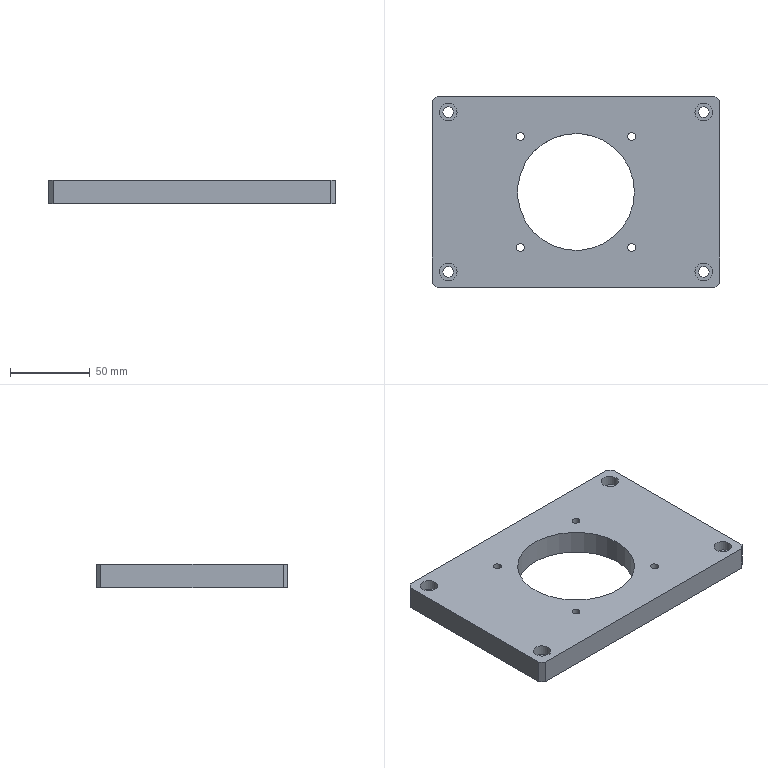Part | NX | 1 solid | 29 faces | box 180 x 120 x 15 mm | volume 255779 mm3 | plane 14 | cylinder 14 | cone 1 | commonest cylinder face diameters 5 x4 6.6 x4 11 x4 2.5 x1 73.2 x1
STEP:
#1=CARTESIAN_POINT('',(-87.,60.,7.5));
#2=VERTEX_POINT('',#1);
#3=CARTESIAN_POINT('',(-90.,57.,7.5));
#4=VERTEX_POINT('',#3);
#5=CARTESIAN_POINT('',(-73.5,73.5,7.5));
#6=DIRECTION('',(-0.7071,-0.7071,0.));
#7=VECTOR('',#6,1000.);
#8=LINE('',#5,#7);
#9=EDGE_CURVE('',#2,#4,#8,.T.);
#10=ORIENTED_EDGE('',*,*,#9,.F.);
#11=CARTESIAN_POINT('',(-87.,60.,-7.5));
#12=VERTEX_POINT('',#11);
#13=CARTESIAN_POINT('',(-87.,60.,7.5));
#14=DIRECTION('',(0.,0.,1.));
#15=VECTOR('',#14,1000.);
#16=LINE('',#13,#15);
#17=EDGE_CURVE('',#12,#2,#16,.T.);
#18=ORIENTED_EDGE('',*,*,#17,.F.);
#19=CARTESIAN_POINT('',(-90.,57.,-7.5));
#20=VERTEX_POINT('',#19);
#21=CARTESIAN_POINT('',(-90.,57.,-7.5));
#22=DIRECTION('',(0.7071,0.7071,0.));
#23=VECTOR('',#22,1000.);
#24=LINE('',#21,#23);
#25=EDGE_CURVE('',#20,#12,#24,.T.);
#26=ORIENTED_EDGE('',*,*,#25,.F.);
#27=CARTESIAN_POINT('',(-90.,57.,7.5));
#28=DIRECTION('',(0.,0.,-1.));
#29=VECTOR('',#28,1000.);
#30=LINE('',#27,#29);
#31=EDGE_CURVE('',#4,#20,#30,.T.);
#32=ORIENTED_EDGE('',*,*,#31,.F.);
#33=EDGE_LOOP('',(#10,#18,#26,#32));
#34=FACE_BOUND('',#33,.T.);
#35=CARTESIAN_POINT('',(-90.,57.,7.5));
#36=DIRECTION('',(0.7071,-0.7071,0.));
#37=DIRECTION('',(0.,0.,-1.));
#38=AXIS2_PLACEMENT_3D('',#35,#36,#37);
#39=PLANE('',#38);
#40=ADVANCED_FACE('',(#34),#39,.F.);
#41=CARTESIAN_POINT('',(90.,57.,7.5));
#42=VERTEX_POINT('',#41);
#43=CARTESIAN_POINT('',(87.,60.,7.5));
#44=VERTEX_POINT('',#43);
#45=CARTESIAN_POINT('',(73.5,73.5,7.5));
#46=DIRECTION('',(-0.7071,0.7071,0.));
#47=VECTOR('',#46,1000.);
#48=LINE('',#45,#47);
#49=EDGE_CURVE('',#42,#44,#48,.T.);
#50=ORIENTED_EDGE('',*,*,#49,.F.);
#51=CARTESIAN_POINT('',(90.,57.,-7.5));
#52=VERTEX_POINT('',#51);
#53=CARTESIAN_POINT('',(90.,57.,7.5));
#54=DIRECTION('',(0.,0.,1.));
#55=VECTOR('',#54,1000.);
#56=LINE('',#53,#55);
#57=EDGE_CURVE('',#52,#42,#56,.T.);
#58=ORIENTED_EDGE('',*,*,#57,.F.);
#59=CARTESIAN_POINT('',(87.,60.,-7.5));
#60=VERTEX_POINT('',#59);
#61=CARTESIAN_POINT('',(87.,60.,-7.5));
#62=DIRECTION('',(0.7071,-0.7071,0.));
#63=VECTOR('',#62,1000.);
#64=LINE('',#61,#63);
#65=EDGE_CURVE('',#60,#52,#64,.T.);
#66=ORIENTED_EDGE('',*,*,#65,.F.);
#67=CARTESIAN_POINT('',(87.,60.,7.5));
#68=DIRECTION('',(0.,0.,-1.));
#69=VECTOR('',#68,1000.);
#70=LINE('',#67,#69);
#71=EDGE_CURVE('',#44,#60,#70,.T.);
#72=ORIENTED_EDGE('',*,*,#71,.F.);
#73=EDGE_LOOP('',(#50,#58,#66,#72));
#74=FACE_BOUND('',#73,.T.);
#75=CARTESIAN_POINT('',(87.,60.,7.5));
#76=DIRECTION('',(-0.7071,-0.7071,0.));
#77=DIRECTION('',(0.,0.,-1.));
#78=AXIS2_PLACEMENT_3D('',#75,#76,#77);
#79=PLANE('',#78);
#80=ADVANCED_FACE('',(#74),#79,.F.);
#81=CARTESIAN_POINT('',(87.,-60.,7.5));
#82=VERTEX_POINT('',#81);
#83=CARTESIAN_POINT('',(90.,-57.,7.5));
#84=VERTEX_POINT('',#83);
#85=CARTESIAN_POINT('',(73.5,-73.5,7.5));
#86=DIRECTION('',(0.7071,0.7071,0.));
#87=VECTOR('',#86,1000.);
#88=LINE('',#85,#87);
#89=EDGE_CURVE('',#82,#84,#88,.T.);
#90=ORIENTED_EDGE('',*,*,#89,.F.);
#91=CARTESIAN_POINT('',(87.,-60.,-7.5));
#92=VERTEX_POINT('',#91);
#93=CARTESIAN_POINT('',(87.,-60.,7.5));
#94=DIRECTION('',(0.,0.,1.));
#95=VECTOR('',#94,1000.);
#96=LINE('',#93,#95);
#97=EDGE_CURVE('',#92,#82,#96,.T.);
#98=ORIENTED_EDGE('',*,*,#97,.F.);
#99=CARTESIAN_POINT('',(90.,-57.,-7.5));
#100=VERTEX_POINT('',#99);
#101=CARTESIAN_POINT('',(90.,-57.,-7.5));
#102=DIRECTION('',(-0.7071,-0.7071,0.));
#103=VECTOR('',#102,1000.);
#104=LINE('',#101,#103);
#105=EDGE_CURVE('',#100,#92,#104,.T.);
#106=ORIENTED_EDGE('',*,*,#105,.F.);
#107=CARTESIAN_POINT('',(90.,-57.,7.5));
#108=DIRECTION('',(0.,0.,-1.));
#109=VECTOR('',#108,1000.);
#110=LINE('',#107,#109);
#111=EDGE_CURVE('',#84,#100,#110,.T.);
#112=ORIENTED_EDGE('',*,*,#111,.F.);
#113=EDGE_LOOP('',(#90,#98,#106,#112));
#114=FACE_BOUND('',#113,.T.);
#115=CARTESIAN_POINT('',(90.,-57.,7.5));
#116=DIRECTION('',(-0.7071,0.7071,0.));
#117=DIRECTION('',(0.,0.,-1.));
#118=AXIS2_PLACEMENT_3D('',#115,#116,#117);
#119=PLANE('',#118);
#120=ADVANCED_FACE('',(#114),#119,.F.);
#121=CARTESIAN_POINT('',(-90.,-57.,7.5));
#122=VERTEX_POINT('',#121);
#123=CARTESIAN_POINT('',(-87.,-60.,7.5));
#124=VERTEX_POINT('',#123);
#125=CARTESIAN_POINT('',(-73.5,-73.5,7.5));
#126=DIRECTION('',(0.7071,-0.7071,0.));
#127=VECTOR('',#126,1000.);
#128=LINE('',#125,#127);
#129=EDGE_CURVE('',#122,#124,#128,.T.);
#130=ORIENTED_EDGE('',*,*,#129,.F.);
#131=CARTESIAN_POINT('',(-90.,-57.,-7.5));
#132=VERTEX_POINT('',#131);
#133=CARTESIAN_POINT('',(-90.,-57.,7.5));
#134=DIRECTION('',(0.,0.,1.));
#135=VECTOR('',#134,1000.);
#136=LINE('',#133,#135);
#137=EDGE_CURVE('',#132,#122,#136,.T.);
#138=ORIENTED_EDGE('',*,*,#137,.F.);
#139=CARTESIAN_POINT('',(-87.,-60.,-7.5));
#140=VERTEX_POINT('',#139);
#141=CARTESIAN_POINT('',(-87.,-60.,-7.5));
#142=DIRECTION('',(-0.7071,0.7071,0.));
#143=VECTOR('',#142,1000.);
#144=LINE('',#141,#143);
#145=EDGE_CURVE('',#140,#132,#144,.T.);
#146=ORIENTED_EDGE('',*,*,#145,.F.);
#147=CARTESIAN_POINT('',(-87.,-60.,7.5));
#148=DIRECTION('',(0.,0.,-1.));
#149=VECTOR('',#148,1000.);
#150=LINE('',#147,#149);
#151=EDGE_CURVE('',#124,#140,#150,.T.);
#152=ORIENTED_EDGE('',*,*,#151,.F.);
#153=EDGE_LOOP('',(#130,#138,#146,#152));
#154=FACE_BOUND('',#153,.T.);
#155=CARTESIAN_POINT('',(-87.,-60.,7.5));
#156=DIRECTION('',(0.7071,0.7071,0.));
#157=DIRECTION('',(0.,0.,-1.));
#158=AXIS2_PLACEMENT_3D('',#155,#156,#157);
#159=PLANE('',#158);
#160=ADVANCED_FACE('',(#154),#159,.F.);
#161=CARTESIAN_POINT('',(-85.5,50.,1.1));
#162=VERTEX_POINT('',#161);
#163=CARTESIAN_POINT('',(-80.,50.,1.1));
#164=DIRECTION('',(0.,0.,1.));
#165=DIRECTION('',(-1.,0.,0.));
#166=AXIS2_PLACEMENT_3D('',#163,#164,#165);
#167=CIRCLE('',#166,5.5);
#168=EDGE_CURVE('',#162,#162,#167,.T.);
#169=ORIENTED_EDGE('',*,*,#168,.T.);
#170=EDGE_LOOP('',(#169));
#171=FACE_BOUND('',#170,.T.);
#172=CARTESIAN_POINT('',(-83.3,50.,1.1));
#173=VERTEX_POINT('',#172);
#174=CARTESIAN_POINT('',(-80.,50.,1.1));
#175=DIRECTION('',(0.,0.,1.));
#176=DIRECTION('',(-1.,0.,0.));
#177=AXIS2_PLACEMENT_3D('',#174,#175,#176);
#178=CIRCLE('',#177,3.3);
#179=EDGE_CURVE('',#173,#173,#178,.T.);
#180=ORIENTED_EDGE('',*,*,#179,.F.);
#181=EDGE_LOOP('',(#180));
#182=FACE_BOUND('',#181,.T.);
#183=CARTESIAN_POINT('',(-76.7,-50.,1.1));
#184=DIRECTION('',(0.,0.,-1.));
#185=DIRECTION('',(-1.,0.,0.));
#186=AXIS2_PLACEMENT_3D('',#183,#184,#185);
#187=PLANE('',#186);
#188=ADVANCED_FACE('',(#171,#182),#187,.F.);
#189=CARTESIAN_POINT('',(74.5,50.,1.1));
#190=VERTEX_POINT('',#189);
#191=CARTESIAN_POINT('',(80.,50.,1.1));
#192=DIRECTION('',(0.,0.,1.));
#193=DIRECTION('',(-1.,0.,0.));
#194=AXIS2_PLACEMENT_3D('',#191,#192,#193);
#195=CIRCLE('',#194,5.5);
#196=EDGE_CURVE('',#190,#190,#195,.T.);
#197=ORIENTED_EDGE('',*,*,#196,.T.);
#198=EDGE_LOOP('',(#197));
#199=FACE_BOUND('',#198,.T.);
#200=CARTESIAN_POINT('',(76.7,50.,1.1));
#201=VERTEX_POINT('',#200);
#202=CARTESIAN_POINT('',(80.,50.,1.1));
#203=DIRECTION('',(0.,0.,1.));
#204=DIRECTION('',(-1.,0.,0.));
#205=AXIS2_PLACEMENT_3D('',#202,#203,#204);
#206=CIRCLE('',#205,3.3);
#207=EDGE_CURVE('',#201,#201,#206,.T.);
#208=ORIENTED_EDGE('',*,*,#207,.F.);
#209=EDGE_LOOP('',(#208));
#210=FACE_BOUND('',#209,.T.);
#211=CARTESIAN_POINT('',(-76.7,-50.,1.1));
#212=DIRECTION('',(0.,0.,-1.));
#213=DIRECTION('',(-1.,0.,0.));
#214=AXIS2_PLACEMENT_3D('',#211,#212,#213);
#215=PLANE('',#214);
#216=ADVANCED_FACE('',(#199,#210),#215,.F.);
#217=CARTESIAN_POINT('',(74.5,-50.,1.1));
#218=VERTEX_POINT('',#217);
#219=CARTESIAN_POINT('',(80.,-50.,1.1));
#220=DIRECTION('',(0.,0.,1.));
#221=DIRECTION('',(-1.,0.,0.));
#222=AXIS2_PLACEMENT_3D('',#219,#220,#221);
#223=CIRCLE('',#222,5.5);
#224=EDGE_CURVE('',#218,#218,#223,.T.);
#225=ORIENTED_EDGE('',*,*,#224,.T.);
#226=EDGE_LOOP('',(#225));
#227=FACE_BOUND('',#226,.T.);
#228=CARTESIAN_POINT('',(76.7,-50.,1.1));
#229=VERTEX_POINT('',#228);
#230=CARTESIAN_POINT('',(80.,-50.,1.1));
#231=DIRECTION('',(0.,0.,1.));
#232=DIRECTION('',(-1.,0.,0.));
#233=AXIS2_PLACEMENT_3D('',#230,#231,#232);
#234=CIRCLE('',#233,3.3);
#235=EDGE_CURVE('',#229,#229,#234,.T.);
#236=ORIENTED_EDGE('',*,*,#235,.F.);
#237=EDGE_LOOP('',(#236));
#238=FACE_BOUND('',#237,.T.);
#239=CARTESIAN_POINT('',(-76.7,-50.,1.1));
#240=DIRECTION('',(0.,0.,-1.));
#241=DIRECTION('',(-1.,0.,0.));
#242=AXIS2_PLACEMENT_3D('',#239,#240,#241);
#243=PLANE('',#242);
#244=ADVANCED_FACE('',(#227,#238),#243,.F.);
#245=CARTESIAN_POINT('',(-74.5,-50.,1.1));
#246=VERTEX_POINT('',#245);
#247=CARTESIAN_POINT('',(-80.,-50.,1.1));
#248=DIRECTION('',(0.,0.,1.));
#249=DIRECTION('',(1.,0.,0.));
#250=AXIS2_PLACEMENT_3D('',#247,#248,#249);
#251=CIRCLE('',#250,5.5);
#252=EDGE_CURVE('',#246,#246,#251,.T.);
#253=ORIENTED_EDGE('',*,*,#252,.T.);
#254=EDGE_LOOP('',(#253));
#255=FACE_BOUND('',#254,.T.);
#256=CARTESIAN_POINT('',(-76.7,-50.,1.1));
#257=VERTEX_POINT('',#256);
#258=CARTESIAN_POINT('',(-80.,-50.,1.1));
#259=DIRECTION('',(0.,0.,1.));
#260=DIRECTION('',(1.,0.,0.));
#261=AXIS2_PLACEMENT_3D('',#258,#259,#260);
#262=CIRCLE('',#261,3.3);
#263=EDGE_CURVE('',#257,#257,#262,.T.);
#264=ORIENTED_EDGE('',*,*,#263,.F.);
#265=EDGE_LOOP('',(#264));
#266=FACE_BOUND('',#265,.T.);
#267=CARTESIAN_POINT('',(-76.7,-50.,1.1));
#268=DIRECTION('',(0.,0.,-1.));
#269=DIRECTION('',(-1.,0.,0.));
#270=AXIS2_PLACEMENT_3D('',#267,#268,#269);
#271=PLANE('',#270);
#272=ADVANCED_FACE('',(#255,#266),#271,.F.);
#273=CARTESIAN_POINT('',(-90.,-60.,-7.5));
#274=DIRECTION('',(1.,0.,0.));
#275=VECTOR('',#274,1000.);
#276=LINE('',#273,#275);
#277=EDGE_CURVE('',#140,#92,#276,.T.);
#278=ORIENTED_EDGE('',*,*,#277,.F.);
#279=ORIENTED_EDGE('',*,*,#145,.T.);
#280=CARTESIAN_POINT('',(-90.,60.,-7.5));
#281=DIRECTION('',(0.,-1.,0.));
#282=VECTOR('',#281,1000.);
#283=LINE('',#280,#282);
#284=EDGE_CURVE('',#20,#132,#283,.T.);
#285=ORIENTED_EDGE('',*,*,#284,.F.);
#286=ORIENTED_EDGE('',*,*,#25,.T.);
#287=CARTESIAN_POINT('',(-90.,60.,-7.5));
#288=DIRECTION('',(-1.,0.,0.));
#289=VECTOR('',#288,1000.);
#290=LINE('',#287,#289);
#291=EDGE_CURVE('',#60,#12,#290,.T.);
#292=ORIENTED_EDGE('',*,*,#291,.F.);
#293=ORIENTED_EDGE('',*,*,#65,.T.);
#294=CARTESIAN_POINT('',(90.,60.,-7.5));
#295=DIRECTION('',(0.,1.,0.));
#296=VECTOR('',#295,1000.);
#297=LINE('',#294,#296);
#298=EDGE_CURVE('',#100,#52,#297,.T.);
#299=ORIENTED_EDGE('',*,*,#298,.F.);
#300=ORIENTED_EDGE('',*,*,#105,.T.);
#301=EDGE_LOOP('',(#278,#279,#285,#286,#292,#293,#299,#300));
#302=FACE_BOUND('',#301,.T.);
#303=CARTESIAN_POINT('',(36.6,0.,-7.5));
#304=VERTEX_POINT('',#303);
#305=CARTESIAN_POINT('',(0.,0.,-7.5));
#306=DIRECTION('',(0.,0.,1.));
#307=DIRECTION('',(1.,0.,0.));
#308=AXIS2_PLACEMENT_3D('',#305,#306,#307);
#309=CIRCLE('',#308,36.6);
#310=EDGE_CURVE('',#304,#304,#309,.T.);
#311=ORIENTED_EDGE('',*,*,#310,.T.);
#312=EDGE_LOOP('',(#311));
#313=FACE_BOUND('',#312,.T.);
#314=CARTESIAN_POINT('',(-76.7,-50.,-7.5));
#315=VERTEX_POINT('',#314);
#316=CARTESIAN_POINT('',(-80.,-50.,-7.5));
#317=DIRECTION('',(0.,0.,1.));
#318=DIRECTION('',(1.,0.,0.));
#319=AXIS2_PLACEMENT_3D('',#316,#317,#318);
#320=CIRCLE('',#319,3.3);
#321=EDGE_CURVE('',#315,#315,#320,.T.);
#322=ORIENTED_EDGE('',*,*,#321,.T.);
#323=EDGE_LOOP('',(#322));
#324=FACE_BOUND('',#323,.T.);
#325=CARTESIAN_POINT('',(83.3,-50.,-7.5));
#326=VERTEX_POINT('',#325);
#327=CARTESIAN_POINT('',(80.,-50.,-7.5));
#328=DIRECTION('',(0.,0.,1.));
#329=DIRECTION('',(1.,0.,0.));
#330=AXIS2_PLACEMENT_3D('',#327,#328,#329);
#331=CIRCLE('',#330,3.3);
#332=EDGE_CURVE('',#326,#326,#331,.T.);
#333=ORIENTED_EDGE('',*,*,#332,.T.);
#334=EDGE_LOOP('',(#333));
#335=FACE_BOUND('',#334,.T.);
#336=CARTESIAN_POINT('',(83.3,50.,-7.5));
#337=VERTEX_POINT('',#336);
#338=CARTESIAN_POINT('',(80.,50.,-7.5));
#339=DIRECTION('',(0.,0.,1.));
#340=DIRECTION('',(1.,0.,0.));
#341=AXIS2_PLACEMENT_3D('',#338,#339,#340);
#342=CIRCLE('',#341,3.3);
#343=EDGE_CURVE('',#337,#337,#342,.T.);
#344=ORIENTED_EDGE('',*,*,#343,.T.);
#345=EDGE_LOOP('',(#344));
#346=FACE_BOUND('',#345,.T.);
#347=CARTESIAN_POINT('',(-76.7,50.,-7.5));
#348=VERTEX_POINT('',#347);
#349=CARTESIAN_POINT('',(-80.,50.,-7.5));
#350=DIRECTION('',(0.,0.,1.));
#351=DIRECTION('',(1.,0.,0.));
#352=AXIS2_PLACEMENT_3D('',#349,#350,#351);
#353=CIRCLE('',#352,3.3);
#354=EDGE_CURVE('',#348,#348,#353,.T.);
#355=ORIENTED_EDGE('',*,*,#354,.T.);
#356=EDGE_LOOP('',(#355));
#357=FACE_BOUND('',#356,.T.);
#358=CARTESIAN_POINT('',(-32.3,-34.8,-7.5));
#359=VERTEX_POINT('',#358);
#360=CARTESIAN_POINT('',(-34.8,-34.8,-7.5));
#361=DIRECTION('',(0.,0.,1.));
#362=DIRECTION('',(1.,0.,0.));
#363=AXIS2_PLACEMENT_3D('',#360,#361,#362);
#364=CIRCLE('',#363,2.5);
#365=EDGE_CURVE('',#359,#359,#364,.T.);
#366=ORIENTED_EDGE('',*,*,#365,.T.);
#367=EDGE_LOOP('',(#366));
#368=FACE_BOUND('',#367,.T.);
#369=CARTESIAN_POINT('',(37.3,-34.8,-7.5));
#370=VERTEX_POINT('',#369);
#371=CARTESIAN_POINT('',(34.8,-34.8,-7.5));
#372=DIRECTION('',(0.,0.,1.));
#373=DIRECTION('',(1.,0.,0.));
#374=AXIS2_PLACEMENT_3D('',#371,#372,#373);
#375=CIRCLE('',#374,2.5);
#376=EDGE_CURVE('',#370,#370,#375,.T.);
#377=ORIENTED_EDGE('',*,*,#376,.T.);
#378=EDGE_LOOP('',(#377));
#379=FACE_BOUND('',#378,.T.);
#380=CARTESIAN_POINT('',(37.3,34.8,-7.5));
#381=VERTEX_POINT('',#380);
#382=CARTESIAN_POINT('',(34.8,34.8,-7.5));
#383=DIRECTION('',(0.,0.,1.));
#384=DIRECTION('',(1.,0.,0.));
#385=AXIS2_PLACEMENT_3D('',#382,#383,#384);
#386=CIRCLE('',#385,2.5);
#387=EDGE_CURVE('',#381,#381,#386,.T.);
#388=ORIENTED_EDGE('',*,*,#387,.T.);
#389=EDGE_LOOP('',(#388));
#390=FACE_BOUND('',#389,.T.);
#391=CARTESIAN_POINT('',(-32.3,34.8,-7.5));
#392=VERTEX_POINT('',#391);
#393=CARTESIAN_POINT('',(-34.8,34.8,-7.5));
#394=DIRECTION('',(0.,0.,1.));
#395=DIRECTION('',(1.,0.,0.));
#396=AXIS2_PLACEMENT_3D('',#393,#394,#395);
#397=CIRCLE('',#396,2.5);
#398=EDGE_CURVE('',#392,#392,#397,.T.);
#399=ORIENTED_EDGE('',*,*,#398,.T.);
#400=EDGE_LOOP('',(#399));
#401=FACE_BOUND('',#400,.T.);
#402=CARTESIAN_POINT('',(0.,0.,-7.5));
#403=DIRECTION('',(0.,0.,1.));
#404=DIRECTION('',(1.,0.,0.));
#405=AXIS2_PLACEMENT_3D('',#402,#403,#404);
#406=PLANE('',#405);
#407=ADVANCED_FACE('',(#302,#313,#324,#335,#346,#357,#368,#379,#390,#401),#406,.F.);
#408=CARTESIAN_POINT('',(-90.,60.,7.5));
#409=DIRECTION('',(0.,-1.,0.));
#410=VECTOR('',#409,1000.);
#411=LINE('',#408,#410);
#412=EDGE_CURVE('',#4,#122,#411,.T.);
#413=ORIENTED_EDGE('',*,*,#412,.T.);
#414=ORIENTED_EDGE('',*,*,#129,.T.);
#415=CARTESIAN_POINT('',(-90.,-60.,7.5));
#416=DIRECTION('',(1.,0.,0.));
#417=VECTOR('',#416,1000.);
#418=LINE('',#415,#417);
#419=EDGE_CURVE('',#124,#82,#418,.T.);
#420=ORIENTED_EDGE('',*,*,#419,.T.);
#421=ORIENTED_EDGE('',*,*,#89,.T.);
#422=CARTESIAN_POINT('',(90.,60.,7.5));
#423=DIRECTION('',(0.,1.,0.));
#424=VECTOR('',#423,1000.);
#425=LINE('',#422,#424);
#426=EDGE_CURVE('',#84,#42,#425,.T.);
#427=ORIENTED_EDGE('',*,*,#426,.T.);
#428=ORIENTED_EDGE('',*,*,#49,.T.);
#429=CARTESIAN_POINT('',(-90.,60.,7.5));
#430=DIRECTION('',(-1.,0.,0.));
#431=VECTOR('',#430,1000.);
#432=LINE('',#429,#431);
#433=EDGE_CURVE('',#44,#2,#432,.T.);
#434=ORIENTED_EDGE('',*,*,#433,.T.);
#435=ORIENTED_EDGE('',*,*,#9,.T.);
#436=EDGE_LOOP('',(#413,#414,#420,#421,#427,#428,#434,#435));
#437=FACE_BOUND('',#436,.T.);
#438=CARTESIAN_POINT('',(36.6,0.,7.5));
#439=VERTEX_POINT('',#438);
#440=CARTESIAN_POINT('',(0.,0.,7.5));
#441=DIRECTION('',(0.,0.,1.));
#442=DIRECTION('',(1.,0.,0.));
#443=AXIS2_PLACEMENT_3D('',#440,#441,#442);
#444=CIRCLE('',#443,36.6);
#445=EDGE_CURVE('',#439,#439,#444,.T.);
#446=ORIENTED_EDGE('',*,*,#445,.F.);
#447=EDGE_LOOP('',(#446));
#448=FACE_BOUND('',#447,.T.);
#449=CARTESIAN_POINT('',(-74.5,-50.,7.5));
#450=VERTEX_POINT('',#449);
#451=CARTESIAN_POINT('',(-80.,-50.,7.5));
#452=DIRECTION('',(0.,0.,1.));
#453=DIRECTION('',(1.,0.,0.));
#454=AXIS2_PLACEMENT_3D('',#451,#452,#453);
#455=CIRCLE('',#454,5.5);
#456=EDGE_CURVE('',#450,#450,#455,.T.);
#457=ORIENTED_EDGE('',*,*,#456,.F.);
#458=EDGE_LOOP('',(#457));
#459=FACE_BOUND('',#458,.T.);
#460=CARTESIAN_POINT('',(85.5,-50.,7.5));
#461=VERTEX_POINT('',#460);
#462=CARTESIAN_POINT('',(80.,-50.,7.5));
#463=DIRECTION('',(0.,0.,1.));
#464=DIRECTION('',(1.,0.,0.));
#465=AXIS2_PLACEMENT_3D('',#462,#463,#464);
#466=CIRCLE('',#465,5.5);
#467=EDGE_CURVE('',#461,#461,#466,.T.);
#468=ORIENTED_EDGE('',*,*,#467,.F.);
#469=EDGE_LOOP('',(#468));
#470=FACE_BOUND('',#469,.T.);
#471=CARTESIAN_POINT('',(85.5,50.,7.5));
#472=VERTEX_POINT('',#471);
#473=CARTESIAN_POINT('',(80.,50.,7.5));
#474=DIRECTION('',(0.,0.,1.));
#475=DIRECTION('',(1.,0.,0.));
#476=AXIS2_PLACEMENT_3D('',#473,#474,#475);
#477=CIRCLE('',#476,5.5);
#478=EDGE_CURVE('',#472,#472,#477,.T.);
#479=ORIENTED_EDGE('',*,*,#478,.F.);
#480=EDGE_LOOP('',(#479));
#481=FACE_BOUND('',#480,.T.);
#482=CARTESIAN_POINT('',(-74.5,50.,7.5));
#483=VERTEX_POINT('',#482);
#484=CARTESIAN_POINT('',(-80.,50.,7.5));
#485=DIRECTION('',(0.,0.,1.));
#486=DIRECTION('',(1.,0.,0.));
#487=AXIS2_PLACEMENT_3D('',#484,#485,#486);
#488=CIRCLE('',#487,5.5);
#489=EDGE_CURVE('',#483,#483,#488,.T.);
#490=ORIENTED_EDGE('',*,*,#489,.F.);
#491=EDGE_LOOP('',(#490));
#492=FACE_BOUND('',#491,.T.);
#493=CARTESIAN_POINT('',(-32.3,-34.8,7.5));
#494=VERTEX_POINT('',#493);
#495=CARTESIAN_POINT('',(-34.8,-34.8,7.5));
#496=DIRECTION('',(0.,0.,1.));
#497=DIRECTION('',(1.,0.,0.));
#498=AXIS2_PLACEMENT_3D('',#495,#496,#497);
#499=CIRCLE('',#498,2.5);
#500=EDGE_CURVE('',#494,#494,#499,.T.);
#501=ORIENTED_EDGE('',*,*,#500,.F.);
#502=EDGE_LOOP('',(#501));
#503=FACE_BOUND('',#502,.T.);
#504=CARTESIAN_POINT('',(37.3,-34.8,7.5));
#505=VERTEX_POINT('',#504);
#506=CARTESIAN_POINT('',(34.8,-34.8,7.5));
#507=DIRECTION('',(0.,0.,1.));
#508=DIRECTION('',(1.,0.,0.));
#509=AXIS2_PLACEMENT_3D('',#506,#507,#508);
#510=CIRCLE('',#509,2.5);
#511=EDGE_CURVE('',#505,#505,#510,.T.);
#512=ORIENTED_EDGE('',*,*,#511,.F.);
#513=EDGE_LOOP('',(#512));
#514=FACE_BOUND('',#513,.T.);
#515=CARTESIAN_POINT('',(37.3,34.8,7.5));
#516=VERTEX_POINT('',#515);
#517=CARTESIAN_POINT('',(34.8,34.8,7.5));
#518=DIRECTION('',(0.,0.,1.));
#519=DIRECTION('',(1.,0.,0.));
#520=AXIS2_PLACEMENT_3D('',#517,#518,#519);
#521=CIRCLE('',#520,2.5);
#522=EDGE_CURVE('',#516,#516,#521,.T.);
#523=ORIENTED_EDGE('',*,*,#522,.F.);
#524=EDGE_LOOP('',(#523));
#525=FACE_BOUND('',#524,.T.);
#526=CARTESIAN_POINT('',(-32.3,34.8,7.5));
#527=VERTEX_POINT('',#526);
#528=CARTESIAN_POINT('',(-34.8,34.8,7.5));
#529=DIRECTION('',(0.,0.,1.));
#530=DIRECTION('',(1.,0.,0.));
#531=AXIS2_PLACEMENT_3D('',#528,#529,#530);
#532=CIRCLE('',#531,2.5);
#533=EDGE_CURVE('',#527,#527,#532,.T.);
#534=ORIENTED_EDGE('',*,*,#533,.F.);
#535=EDGE_LOOP('',(#534));
#536=FACE_BOUND('',#535,.T.);
#537=CARTESIAN_POINT('',(0.,0.,7.5));
#538=DIRECTION('',(0.,0.,1.));
#539=DIRECTION('',(1.,0.,0.));
#540=AXIS2_PLACEMENT_3D('',#537,#538,#539);
#541=PLANE('',#540);
#542=ADVANCED_FACE('',(#437,#448,#459,#470,#481,#492,#503,#514,#525,#536),#541,.T.);
#543=ORIENTED_EDGE('',*,*,#419,.F.);
#544=ORIENTED_EDGE('',*,*,#151,.T.);
#545=ORIENTED_EDGE('',*,*,#277,.T.);
#546=ORIENTED_EDGE('',*,*,#97,.T.);
#547=EDGE_LOOP('',(#543,#544,#545,#546));
#548=FACE_BOUND('',#547,.T.);
#549=CARTESIAN_POINT('',(-90.,-60.,7.5));
#550=DIRECTION('',(0.,1.,0.));
#551=DIRECTION('',(0.,0.,1.));
#552=AXIS2_PLACEMENT_3D('',#549,#550,#551);
#553=PLANE('',#552);
#554=ADVANCED_FACE('',(#548),#553,.F.);
#555=ORIENTED_EDGE('',*,*,#284,.T.);
#556=ORIENTED_EDGE('',*,*,#137,.T.);
#557=ORIENTED_EDGE('',*,*,#412,.F.);
#558=ORIENTED_EDGE('',*,*,#31,.T.);
#559=EDGE_LOOP('',(#555,#556,#557,#558));
#560=FACE_BOUND('',#559,.T.);
#561=CARTESIAN_POINT('',(-90.,60.,7.5));
#562=DIRECTION('',(1.,0.,0.));
#563=DIRECTION('',(0.,1.,0.));
#564=AXIS2_PLACEMENT_3D('',#561,#562,#563);
#565=PLANE('',#564);
#566=ADVANCED_FACE('',(#560),#565,.F.);
#567=ORIENTED_EDGE('',*,*,#433,.F.);
#568=ORIENTED_EDGE('',*,*,#71,.T.);
#569=ORIENTED_EDGE('',*,*,#291,.T.);
#570=ORIENTED_EDGE('',*,*,#17,.T.);
#571=EDGE_LOOP('',(#567,#568,#569,#570));
#572=FACE_BOUND('',#571,.T.);
#573=CARTESIAN_POINT('',(-15.5,60.,1.25));
#574=VERTEX_POINT('',#573);
#575=CARTESIAN_POINT('',(-15.5,60.,0.));
#576=DIRECTION('',(0.,1.,0.));
#577=DIRECTION('',(0.,0.,1.));
#578=AXIS2_PLACEMENT_3D('',#575,#576,#577);
#579=CIRCLE('',#578,1.25);
#580=EDGE_CURVE('',#574,#574,#579,.T.);
#581=ORIENTED_EDGE('',*,*,#580,.F.);
#582=EDGE_LOOP('',(#581));
#583=FACE_BOUND('',#582,.T.);
#584=CARTESIAN_POINT('',(-90.,60.,7.5));
#585=DIRECTION('',(0.,-1.,0.));
#586=DIRECTION('',(0.,0.,-1.));
#587=AXIS2_PLACEMENT_3D('',#584,#585,#586);
#588=PLANE('',#587);
#589=ADVANCED_FACE('',(#572,#583),#588,.F.);
#590=ORIENTED_EDGE('',*,*,#426,.F.);
#591=ORIENTED_EDGE('',*,*,#111,.T.);
#592=ORIENTED_EDGE('',*,*,#298,.T.);
#593=ORIENTED_EDGE('',*,*,#57,.T.);
#594=EDGE_LOOP('',(#590,#591,#592,#593));
#595=FACE_BOUND('',#594,.T.);
#596=CARTESIAN_POINT('',(90.,60.,7.5));
#597=DIRECTION('',(-1.,0.,0.));
#598=DIRECTION('',(0.,-1.,0.));
#599=AXIS2_PLACEMENT_3D('',#596,#597,#598);
#600=PLANE('',#599);
#601=ADVANCED_FACE('',(#595),#600,.F.);
#602=ORIENTED_EDGE('',*,*,#310,.F.);
#603=EDGE_LOOP('',(#602));
#604=FACE_BOUND('',#603,.T.);
#605=ORIENTED_EDGE('',*,*,#445,.T.);
#606=EDGE_LOOP('',(#605));
#607=FACE_BOUND('',#606,.T.);
#608=CARTESIAN_POINT('',(0.,0.,-7.5));
#609=DIRECTION('',(0.,0.,1.));
#610=DIRECTION('',(1.,0.,0.));
#611=AXIS2_PLACEMENT_3D('',#608,#609,#610);
#612=CYLINDRICAL_SURFACE('',#611,36.6);
#613=ADVANCED_FACE('',(#604,#607),#612,.F.);
#614=ORIENTED_EDGE('',*,*,#321,.F.);
#615=EDGE_LOOP('',(#614));
#616=FACE_BOUND('',#615,.T.);
#617=ORIENTED_EDGE('',*,*,#263,.T.);
#618=EDGE_LOOP('',(#617));
#619=FACE_BOUND('',#618,.T.);
#620=CARTESIAN_POINT('',(-80.,-50.,7.5));
#621=DIRECTION('',(0.,0.,1.));
#622=DIRECTION('',(1.,0.,0.));
#623=AXIS2_PLACEMENT_3D('',#620,#621,#622);
#624=CYLINDRICAL_SURFACE('',#623,3.3);
#625=ADVANCED_FACE('',(#616,#619),#624,.F.);
#626=ORIENTED_EDGE('',*,*,#252,.F.);
#627=EDGE_LOOP('',(#626));
#628=FACE_BOUND('',#627,.T.);
#629=ORIENTED_EDGE('',*,*,#456,.T.);
#630=EDGE_LOOP('',(#629));
#631=FACE_BOUND('',#630,.T.);
#632=CARTESIAN_POINT('',(-80.,-50.,7.5));
#633=DIRECTION('',(0.,0.,1.));
#634=DIRECTION('',(1.,0.,0.));
#635=AXIS2_PLACEMENT_3D('',#632,#633,#634);
#636=CYLINDRICAL_SURFACE('',#635,5.5);
#637=ADVANCED_FACE('',(#628,#631),#636,.F.);
#638=ORIENTED_EDGE('',*,*,#332,.F.);
#639=EDGE_LOOP('',(#638));
#640=FACE_BOUND('',#639,.T.);
#641=ORIENTED_EDGE('',*,*,#235,.T.);
#642=EDGE_LOOP('',(#641));
#643=FACE_BOUND('',#642,.T.);
#644=CARTESIAN_POINT('',(80.,-50.,7.5));
#645=DIRECTION('',(0.,0.,1.));
#646=DIRECTION('',(1.,0.,0.));
#647=AXIS2_PLACEMENT_3D('',#644,#645,#646);
#648=CYLINDRICAL_SURFACE('',#647,3.3);
#649=ADVANCED_FACE('',(#640,#643),#648,.F.);
#650=ORIENTED_EDGE('',*,*,#224,.F.);
#651=EDGE_LOOP('',(#650));
#652=FACE_BOUND('',#651,.T.);
#653=ORIENTED_EDGE('',*,*,#467,.T.);
#654=EDGE_LOOP('',(#653));
#655=FACE_BOUND('',#654,.T.);
#656=CARTESIAN_POINT('',(80.,-50.,7.5));
#657=DIRECTION('',(0.,0.,1.));
#658=DIRECTION('',(1.,0.,0.));
#659=AXIS2_PLACEMENT_3D('',#656,#657,#658);
#660=CYLINDRICAL_SURFACE('',#659,5.5);
#661=ADVANCED_FACE('',(#652,#655),#660,.F.);
#662=ORIENTED_EDGE('',*,*,#343,.F.);
#663=EDGE_LOOP('',(#662));
#664=FACE_BOUND('',#663,.T.);
#665=ORIENTED_EDGE('',*,*,#207,.T.);
#666=EDGE_LOOP('',(#665));
#667=FACE_BOUND('',#666,.T.);
#668=CARTESIAN_POINT('',(80.,50.,7.5));
#669=DIRECTION('',(0.,0.,1.));
#670=DIRECTION('',(1.,0.,0.));
#671=AXIS2_PLACEMENT_3D('',#668,#669,#670);
#672=CYLINDRICAL_SURFACE('',#671,3.3);
#673=ADVANCED_FACE('',(#664,#667),#672,.F.);
#674=ORIENTED_EDGE('',*,*,#196,.F.);
#675=EDGE_LOOP('',(#674));
#676=FACE_BOUND('',#675,.T.);
#677=ORIENTED_EDGE('',*,*,#478,.T.);
#678=EDGE_LOOP('',(#677));
#679=FACE_BOUND('',#678,.T.);
#680=CARTESIAN_POINT('',(80.,50.,7.5));
#681=DIRECTION('',(0.,0.,1.));
#682=DIRECTION('',(1.,0.,0.));
#683=AXIS2_PLACEMENT_3D('',#680,#681,#682);
#684=CYLINDRICAL_SURFACE('',#683,5.5);
#685=ADVANCED_FACE('',(#676,#679),#684,.F.);
#686=ORIENTED_EDGE('',*,*,#354,.F.);
#687=EDGE_LOOP('',(#686));
#688=FACE_BOUND('',#687,.T.);
#689=ORIENTED_EDGE('',*,*,#179,.T.);
#690=EDGE_LOOP('',(#689));
#691=FACE_BOUND('',#690,.T.);
#692=CARTESIAN_POINT('',(-80.,50.,7.5));
#693=DIRECTION('',(0.,0.,1.));
#694=DIRECTION('',(1.,0.,0.));
#695=AXIS2_PLACEMENT_3D('',#692,#693,#694);
#696=CYLINDRICAL_SURFACE('',#695,3.3);
#697=ADVANCED_FACE('',(#688,#691),#696,.F.);
#698=ORIENTED_EDGE('',*,*,#168,.F.);
#699=EDGE_LOOP('',(#698));
#700=FACE_BOUND('',#699,.T.);
#701=ORIENTED_EDGE('',*,*,#489,.T.);
#702=EDGE_LOOP('',(#701));
#703=FACE_BOUND('',#702,.T.);
#704=CARTESIAN_POINT('',(-80.,50.,7.5));
#705=DIRECTION('',(0.,0.,1.));
#706=DIRECTION('',(1.,0.,0.));
#707=AXIS2_PLACEMENT_3D('',#704,#705,#706);
#708=CYLINDRICAL_SURFACE('',#707,5.5);
#709=ADVANCED_FACE('',(#700,#703),#708,.F.);
#710=ORIENTED_EDGE('',*,*,#365,.F.);
#711=EDGE_LOOP('',(#710));
#712=FACE_BOUND('',#711,.T.);
#713=ORIENTED_EDGE('',*,*,#500,.T.);
#714=EDGE_LOOP('',(#713));
#715=FACE_BOUND('',#714,.T.);
#716=CARTESIAN_POINT('',(-34.8,-34.8,7.5));
#717=DIRECTION('',(0.,0.,1.));
#718=DIRECTION('',(1.,0.,0.));
#719=AXIS2_PLACEMENT_3D('',#716,#717,#718);
#720=CYLINDRICAL_SURFACE('',#719,2.5);
#721=ADVANCED_FACE('',(#712,#715),#720,.F.);
#722=ORIENTED_EDGE('',*,*,#376,.F.);
#723=EDGE_LOOP('',(#722));
#724=FACE_BOUND('',#723,.T.);
#725=ORIENTED_EDGE('',*,*,#511,.T.);
#726=EDGE_LOOP('',(#725));
#727=FACE_BOUND('',#726,.T.);
#728=CARTESIAN_POINT('',(34.8,-34.8,7.5));
#729=DIRECTION('',(0.,0.,1.));
#730=DIRECTION('',(1.,0.,0.));
#731=AXIS2_PLACEMENT_3D('',#728,#729,#730);
#732=CYLINDRICAL_SURFACE('',#731,2.5);
#733=ADVANCED_FACE('',(#724,#727),#732,.F.);
#734=ORIENTED_EDGE('',*,*,#387,.F.);
#735=EDGE_LOOP('',(#734));
#736=FACE_BOUND('',#735,.T.);
#737=ORIENTED_EDGE('',*,*,#522,.T.);
#738=EDGE_LOOP('',(#737));
#739=FACE_BOUND('',#738,.T.);
#740=CARTESIAN_POINT('',(34.8,34.8,7.5));
#741=DIRECTION('',(0.,0.,1.));
#742=DIRECTION('',(1.,0.,0.));
#743=AXIS2_PLACEMENT_3D('',#740,#741,#742);
#744=CYLINDRICAL_SURFACE('',#743,2.5);
#745=ADVANCED_FACE('',(#736,#739),#744,.F.);
#746=ORIENTED_EDGE('',*,*,#398,.F.);
#747=EDGE_LOOP('',(#746));
#748=FACE_BOUND('',#747,.T.);
#749=ORIENTED_EDGE('',*,*,#533,.T.);
#750=EDGE_LOOP('',(#749));
#751=FACE_BOUND('',#750,.T.);
#752=CARTESIAN_POINT('',(-34.8,34.8,7.5));
#753=DIRECTION('',(0.,0.,1.));
#754=DIRECTION('',(1.,0.,0.));
#755=AXIS2_PLACEMENT_3D('',#752,#753,#754);
#756=CYLINDRICAL_SURFACE('',#755,2.5);
#757=ADVANCED_FACE('',(#748,#751),#756,.F.);
#758=CARTESIAN_POINT('',(-15.5,52.5,1.25));
#759=VERTEX_POINT('',#758);
#760=CARTESIAN_POINT('',(-15.5,52.5,0.));
#761=DIRECTION('',(0.,1.,0.));
#762=DIRECTION('',(0.,0.,1.));
#763=AXIS2_PLACEMENT_3D('',#760,#761,#762);
#764=CIRCLE('',#763,1.25);
#765=EDGE_CURVE('',#759,#759,#764,.T.);
#766=ORIENTED_EDGE('',*,*,#765,.T.);
#767=EDGE_LOOP('',(#766));
#768=FACE_BOUND('',#767,.T.);
#769=CARTESIAN_POINT('',(-15.5,51.749,0.));
#770=VERTEX_POINT('',#769);
#771=VERTEX_LOOP('',#770);
#772=FACE_BOUND('',#771,.T.);
#773=CARTESIAN_POINT('',(-15.5,52.5,0.));
#774=DIRECTION('',(0.,1.,0.));
#775=DIRECTION('',(0.,0.,1.));
#776=AXIS2_PLACEMENT_3D('',#773,#774,#775);
#777=CONICAL_SURFACE('',#776,1.25,1.03);
#778=ADVANCED_FACE('',(#768,#772),#777,.F.);
#779=ORIENTED_EDGE('',*,*,#765,.F.);
#780=EDGE_LOOP('',(#779));
#781=FACE_BOUND('',#780,.T.);
#782=ORIENTED_EDGE('',*,*,#580,.T.);
#783=EDGE_LOOP('',(#782));
#784=FACE_BOUND('',#783,.T.);
#785=CARTESIAN_POINT('',(-15.5,60.,0.));
#786=DIRECTION('',(0.,1.,0.));
#787=DIRECTION('',(0.,0.,1.));
#788=AXIS2_PLACEMENT_3D('',#785,#786,#787);
#789=CYLINDRICAL_SURFACE('',#788,1.25);
#790=ADVANCED_FACE('',(#781,#784),#789,.F.);
#791=CLOSED_SHELL('',(#40,#80,#120,#160,#188,#216,#244,#272,#407,#542,#554,#566,#589,#601,#613,#625,#637,#649,#661,#673,#685,#697,#709,#721,#733,#745,#757,#778,#790));
#792=MANIFOLD_SOLID_BREP('',#791);
#793=(LENGTH_UNIT()NAMED_UNIT(*)SI_UNIT(.MILLI.,.METRE.));
#794=UNCERTAINTY_MEASURE_WITH_UNIT(LENGTH_MEASURE(0.00001),#793,'','');
#795=(NAMED_UNIT(*)PLANE_ANGLE_UNIT()SI_UNIT($,.RADIAN.));
#796=(NAMED_UNIT(*)SI_UNIT($,.STERADIAN.)SOLID_ANGLE_UNIT());
#797=(GEOMETRIC_REPRESENTATION_CONTEXT(3)GLOBAL_UNCERTAINTY_ASSIGNED_CONTEXT((#794))GLOBAL_UNIT_ASSIGNED_CONTEXT((#793,#795,#796))REPRESENTATION_CONTEXT('',''));
#798=ADVANCED_BREP_SHAPE_REPRESENTATION('',(#792),#797);